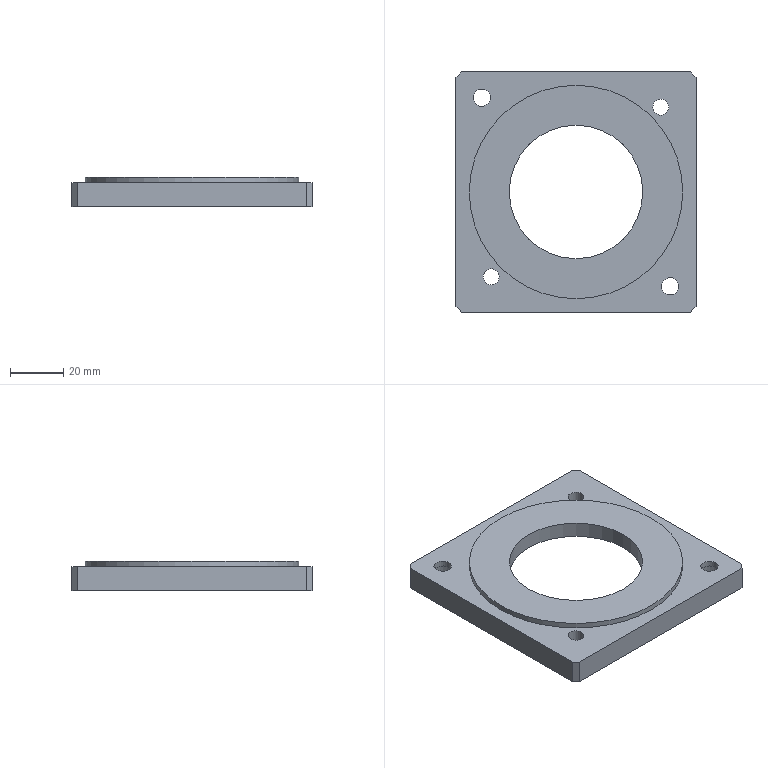NC program | NX | posted with a generic post | part box 90 x 90 x 11 mm
Whole program:
N10 G17 G21 G94 G90
(FLOOR_WALL_COPY , TOOL : D50)
N12 T15 M6
N14 G54
N16 G17 G0 G90 X-73. Y44.997 S6500 M3
N18 G43 Z30. H15
N20 Z6.
N22 G94 G1 Z3. F1250.
N24 X-70.
N26 X70.
N28 Y9.999
N30 X-70.
N32 Y-25.
N34 X70.
N36 X73.
N38 Z6.
N40 G0 Z30.
N42 X-73. Y44.997
N44 Z5.
N46 G1 Z2.
N48 X-70.
N50 X70.
N52 Y9.999
N54 X-70.
N56 Y-25.
N58 X70.
N60 X73.
N62 Z5.
N64 G0 Z30.
N66 X-73. Y44.997
N68 Z4.
N70 G1 Z1.
N72 X-70.
N74 X70.
N76 Y9.999
N78 X-70.
N80 Y-25.
N82 X70.
N84 X73.
N86 Z4.
N88 G0 Z30.
N90 X-73. Y44.997
N92 Z3.
N94 G1 Z0.
N96 X-70.
N98 X70.
N100 Y9.999
N102 X-70.
N104 Y-25.
N106 X70.
N108 X73.
N110 Z3.
N112 G0 Z30.
N114 M5
(HOLE_MILLING_COPY , TOOL : D10)
N116 T10 M6
N118 G54
N120 G17 G0 G90 X-16.272 Y2.731 S9500 M3
N122 G43 Z30. H10
N124 Z0.5
N126 G94 G3 X-19.5 Y0. R2.769 F3000.
N128 X2.444 Y-19.346 Z-4.9 R19.5
N130 X19.465 Y2.597 R19.637
N132 X-2.494 Y19.743 R19.763
N134 X-19.948 Y-2.465 R19.972
N136 X2.544 Y-20.14 R20.227
N138 X20.345 Y2.515 R20.372
N140 X-2.594 Y20.537 R20.627
N142 X-20.742 Y-2.565 R20.772
N144 X2.645 Y-20.934 R21.027
N146 X21.139 Y2.615 R21.172
N148 X-2.695 Y21.33 R21.427
N150 X-21.535 Y-2.665 R21.572
N152 X2.745 Y-21.727 R21.827
N154 X21.932 Y2.716 R21.972
N156 X-2.795 Y22.124 R22.227
N158 X-22.329 Y-2.766 R22.372
N160 X2.845 Y-22.521 R22.627
N162 X22.726 Y2.816 R22.772
N164 X-2.895 Y22.918 R23.027
N166 X-23.123 Y-2.866 R23.172
N168 X2.945 Y-23.315 R23.427
N170 X23.52 Y2.916 R23.572
N172 X-2.995 Y23.712 R23.827
N174 X-23.917 Y-2.966 R23.972
N176 X3.046 Y-24.108 R24.227
N178 X24.313 Y3.016 R24.372
N180 X-3.096 Y24.505 R24.627
N182 X-24.71 Y-3.067 R24.772
N184 X3.146 Y-24.902 R25.027
N186 X25.107 Y3.117 R25.172
N188 X-3.196 Y25.299 R25.427
N190 X-25.504 Y-3.167 R25.572
N192 X3.246 Y-25.696 R25.827
N194 X25.901 Y3.217 R25.972
N196 X-3.296 Y26.093 R26.227
N198 X-26.298 Y-3.267 R26.372
N200 X3.346 Y-26.489 R26.627
N202 X26.694 Y3.317 R26.772
N204 X-3.397 Y26.886 R27.027
N206 X-27.091 Y-3.367 R27.172
N208 X3.447 Y-27.283 R27.427
N210 X27.488 Y3.417 R27.572
N212 X-3.497 Y27.68 R27.827
N214 X-27.885 Y-3.468 R27.972
N216 X3.547 Y-28.077 R28.227
N218 X28.282 Y3.518 R28.372
N220 X-3.597 Y28.474 R28.627
N222 X-28.679 Y-3.568 R28.772
N224 X3.647 Y-28.871 R29.027
N226 X29.076 Y3.618 R29.172
N228 X-3.697 Y29.267 R29.427
N230 X-29.512 Y-3.865 R29.636
N232 X3.747 Y-29.664 R29.764
N234 X29.664 Y3.747 R29.9
N236 X3.747 Y-29.664 R-29.9
N238 X10.477 Y-12.747 R10.397
N240 G0 Z30.
(FLOOR_WALL_1_COPY , TOOL : D10)
N242 X-0.985 Y-28.574
N244 Z-3.5
N246 G1 Z-5. F1250.
N248 G3 X0. Y-29.4 R1.
N250 X29.4 Y0. R29.4
N252 X0. Y-29.4 R-29.4
N254 G1 X-0.985 Y-29.074
N256 G3 X0. Y-29.9 R1.
N258 X29.9 Y0. R29.9
N260 X0. Y-29.9 R-29.9
N262 X0.985 Y-29.074 R1.
N264 G1 X1.107 Y-28.378
N266 Z-3.5
N268 G0 Z30.
N270 M5
(HOLE_MILLING , TOOL : D6)
N272 T06 M6
N274 G54
N276 G17 G0 G90 X-35.355 Y-35.355 S9500 M3
N278 G43 Z30. H6
N280 Z0.5
N282 G94 G3 X-36.605 Y-34.105 R1.25 F1400.
N284 X-37.855 Y-35.355 R1.25
N286 X-37.855 Y-35.355 Z0. I2.5 J0.
N288 X-37.855 Y-35.355 Z-0.5 I2.5 J0.
N290 X-37.855 Y-35.355 Z-1. I2.5 J0.
N292 X-37.855 Y-35.355 Z-1.5 I2.5 J0.
N294 X-37.855 Y-35.355 Z-2. I2.5 J0.
N296 X-37.855 Y-35.355 Z-2.5 I2.5 J0.
N298 X-37.855 Y-35.355 Z-3. I2.5 J0.
N300 X-37.855 Y-35.355 Z-3.5 I2.5 J0.
N302 X-37.855 Y-35.355 Z-4. I2.5 J0.
N304 X-37.855 Y-35.355 Z-4.5 I2.5 J0.
N306 X-37.855 Y-35.355 Z-5. I2.5 J0.
N308 X-37.855 Y-35.355 Z-5.5 I2.5 J0.
N310 X-37.855 Y-35.355 Z-6. I2.5 J0.
N312 X-37.855 Y-35.355 Z-6.5 I2.5 J0.
N314 X-33.333 Y-33.886 Z-6.8 R-2.5
N316 X-36.825 Y-33.333 R2.5
N318 X-33.333 Y-33.886 R-2.5
N320 X-35.079 Y-33.609 R1.25
N322 X-35.355 Y-35.355 R1.25
N324 G0 Z30.
N326 X35.355 Y35.355
N328 Z0.5
N330 G3 X34.105 Y36.605 R1.25
N332 X32.855 Y35.355 R1.25
N334 X32.855 Y35.355 Z0. I2.5 J0.
N336 X32.855 Y35.355 Z-0.5 I2.5 J0.
N338 X32.855 Y35.355 Z-1. I2.5 J0.
N340 X32.855 Y35.355 Z-1.5 I2.5 J0.
N342 X32.855 Y35.355 Z-2. I2.5 J0.
N344 X32.855 Y35.355 Z-2.5 I2.5 J0.
N346 X32.855 Y35.355 Z-3. I2.5 J0.
N348 X32.855 Y35.355 Z-3.5 I2.5 J0.
N350 X32.855 Y35.355 Z-4. I2.5 J0.
N352 X32.855 Y35.355 Z-4.5 I2.5 J0.
N354 X32.855 Y35.355 Z-5. I2.5 J0.
N356 X32.855 Y35.355 Z-5.5 I2.5 J0.
N358 X32.855 Y35.355 Z-6. I2.5 J0.
N360 X32.855 Y35.355 Z-6.5 I2.5 J0.
N362 X37.378 Y36.825 Z-6.8 R-2.5
N364 X33.886 Y37.378 R2.5
N366 X37.378 Y36.825 R-2.5
N368 X35.632 Y37.101 R1.25
N370 X35.355 Y35.355 R1.25
N372 G0 Z30.
N374 M5
(ZLEVEL_PROFILE_COPY_1_COPY_COPY_COPY_COPY_2_COPY_COPY_1 , TOOL : D6A45)
N376 T07 M6
N378 G54
N380 G17 G0 G90 X-32.825 Y1.049 S7000 M3
N382 G43 Z30. H7
N384 Z-1.
N386 G94 G1 X-33.741 Y0.52 F1000.
N388 G3 X-34.041 Y0. R0.6
N390 X0. Y-34.041 R34.041
N392 X-34.041 Y0. R-34.041
N394 X-33.741 Y-0.52 R0.6
N396 G1 X-32.825 Y-1.049
N398 G0 Z30.
N400 X31.579 Y-32.626
N402 Z-1.
N404 G1 X31.3 Y-33.561
N406 G3 X31.82 Y-33.861 R0.6
N408 X33.861 Y-31.82 R2.041
N410 X31.82 Y-33.861 R-2.041
N412 X32.339 Y-33.561 R0.6
N414 G1 X32.06 Y-32.626
N416 G0 Z30.
N418 X-32.626 Y32.06
N420 Z-1.
N422 G1 X-33.561 Y32.339
N424 G3 X-33.861 Y31.82 R0.6
N426 X-31.82 Y29.778 R2.041
N428 X-33.861 Y31.82 R-2.041
N430 X-33.561 Y31.3 R0.6
N432 G1 X-32.626 Y31.579
N434 G0 Z30.
N436 X-38.489 Y-34.196
N438 Z-1.
N440 G1 X-39.597 Y-34.836
N442 G3 X-39.897 Y-35.355 R0.6
N444 X-35.355 Y-39.897 R4.541
N446 X-39.897 Y-35.355 R-4.541
N448 X-39.597 Y-35.875 R0.6
N450 G1 X-38.489 Y-36.514
N452 G0 Z30.
N454 X36.514 Y38.489
N456 Z-1.
N458 G1 X35.875 Y39.597
N460 G3 X35.355 Y39.897 R0.6
N462 X30.814 Y35.355 R4.541
N464 X35.355 Y39.897 R-4.541
N466 X34.836 Y39.597 R0.6
N468 G1 X34.196 Y38.489
N470 G0 Z30.
N472 X-43.911 Y46.955
N474 Z-1.
N476 G1 X-43.509 Y46.259
N478 G3 X-42.99 Y45.959 R0.6
N480 G1 X42.99
N482 G2 X43.685 Y45.67 R0.984
N484 G1 X45.67 Y43.685
N486 G2 X45.959 Y42.99 R0.984
N488 G1 Y-42.99
N490 G2 X45.67 Y-43.685 R0.984
N492 G1 X43.685 Y-45.67
N494 G2 X42.99 Y-45.959 R0.984
N496 G1 X-42.99
N498 G2 X-43.685 Y-45.67 R0.984
N500 G1 X-45.67 Y-43.685
N502 G2 X-45.959 Y-42.99 R0.984
N504 G1 Y42.99
N506 G2 X-45.67 Y43.685 R0.984
N508 G1 X-43.685 Y45.67
N510 G2 X-42.99 Y45.959 R0.984
N512 G3 X-42.47 Y46.259 R0.6
N514 G1 X-41.95 Y47.159
N516 G0 Z30.
(ZLEVEL_PROFILE_COPY_1_COPY_COPY_COPY_COPY_2_COPY_COPY_1_COPY , TOOL : D6A45)
N518 X-22.817 Y1.053
N520 Z-6.
N522 G1 X-23.741 Y0.52
N524 G3 X-24.041 Y0. R0.6
N526 X0. Y-24.041 R24.041
N528 X-24.041 Y0. R-24.041
N530 X-23.741 Y-0.52 R0.6
N532 G1 X-22.817 Y-1.053
N534 G0 Z30.
N536 M5
(刀补10_COPY , TOOL : D10)
N538 T10 M6
N540 G54
N542 G17 G0 G90 X-1.107 Y-28.328 S9500 M3
N544 G43 Z30. H10
N546 Z-3.5
N548 G94 G1 Z-5. F1250.
N550 G41 Y-28.428 D10
N552 X-0.985 Y-29.124
N554 G3 X0. Y-29.95 R1.
N556 X29.95 Y0. R29.95
N558 X0. Y-29.95 R-29.95
N560 X0.985 Y-29.124 R1.
N562 G1 X1.107 Y-28.428
N564 G40
N566 Y-28.328
N568 Z-3.5
N570 G0 Z30.
N572 M5
N574 M2